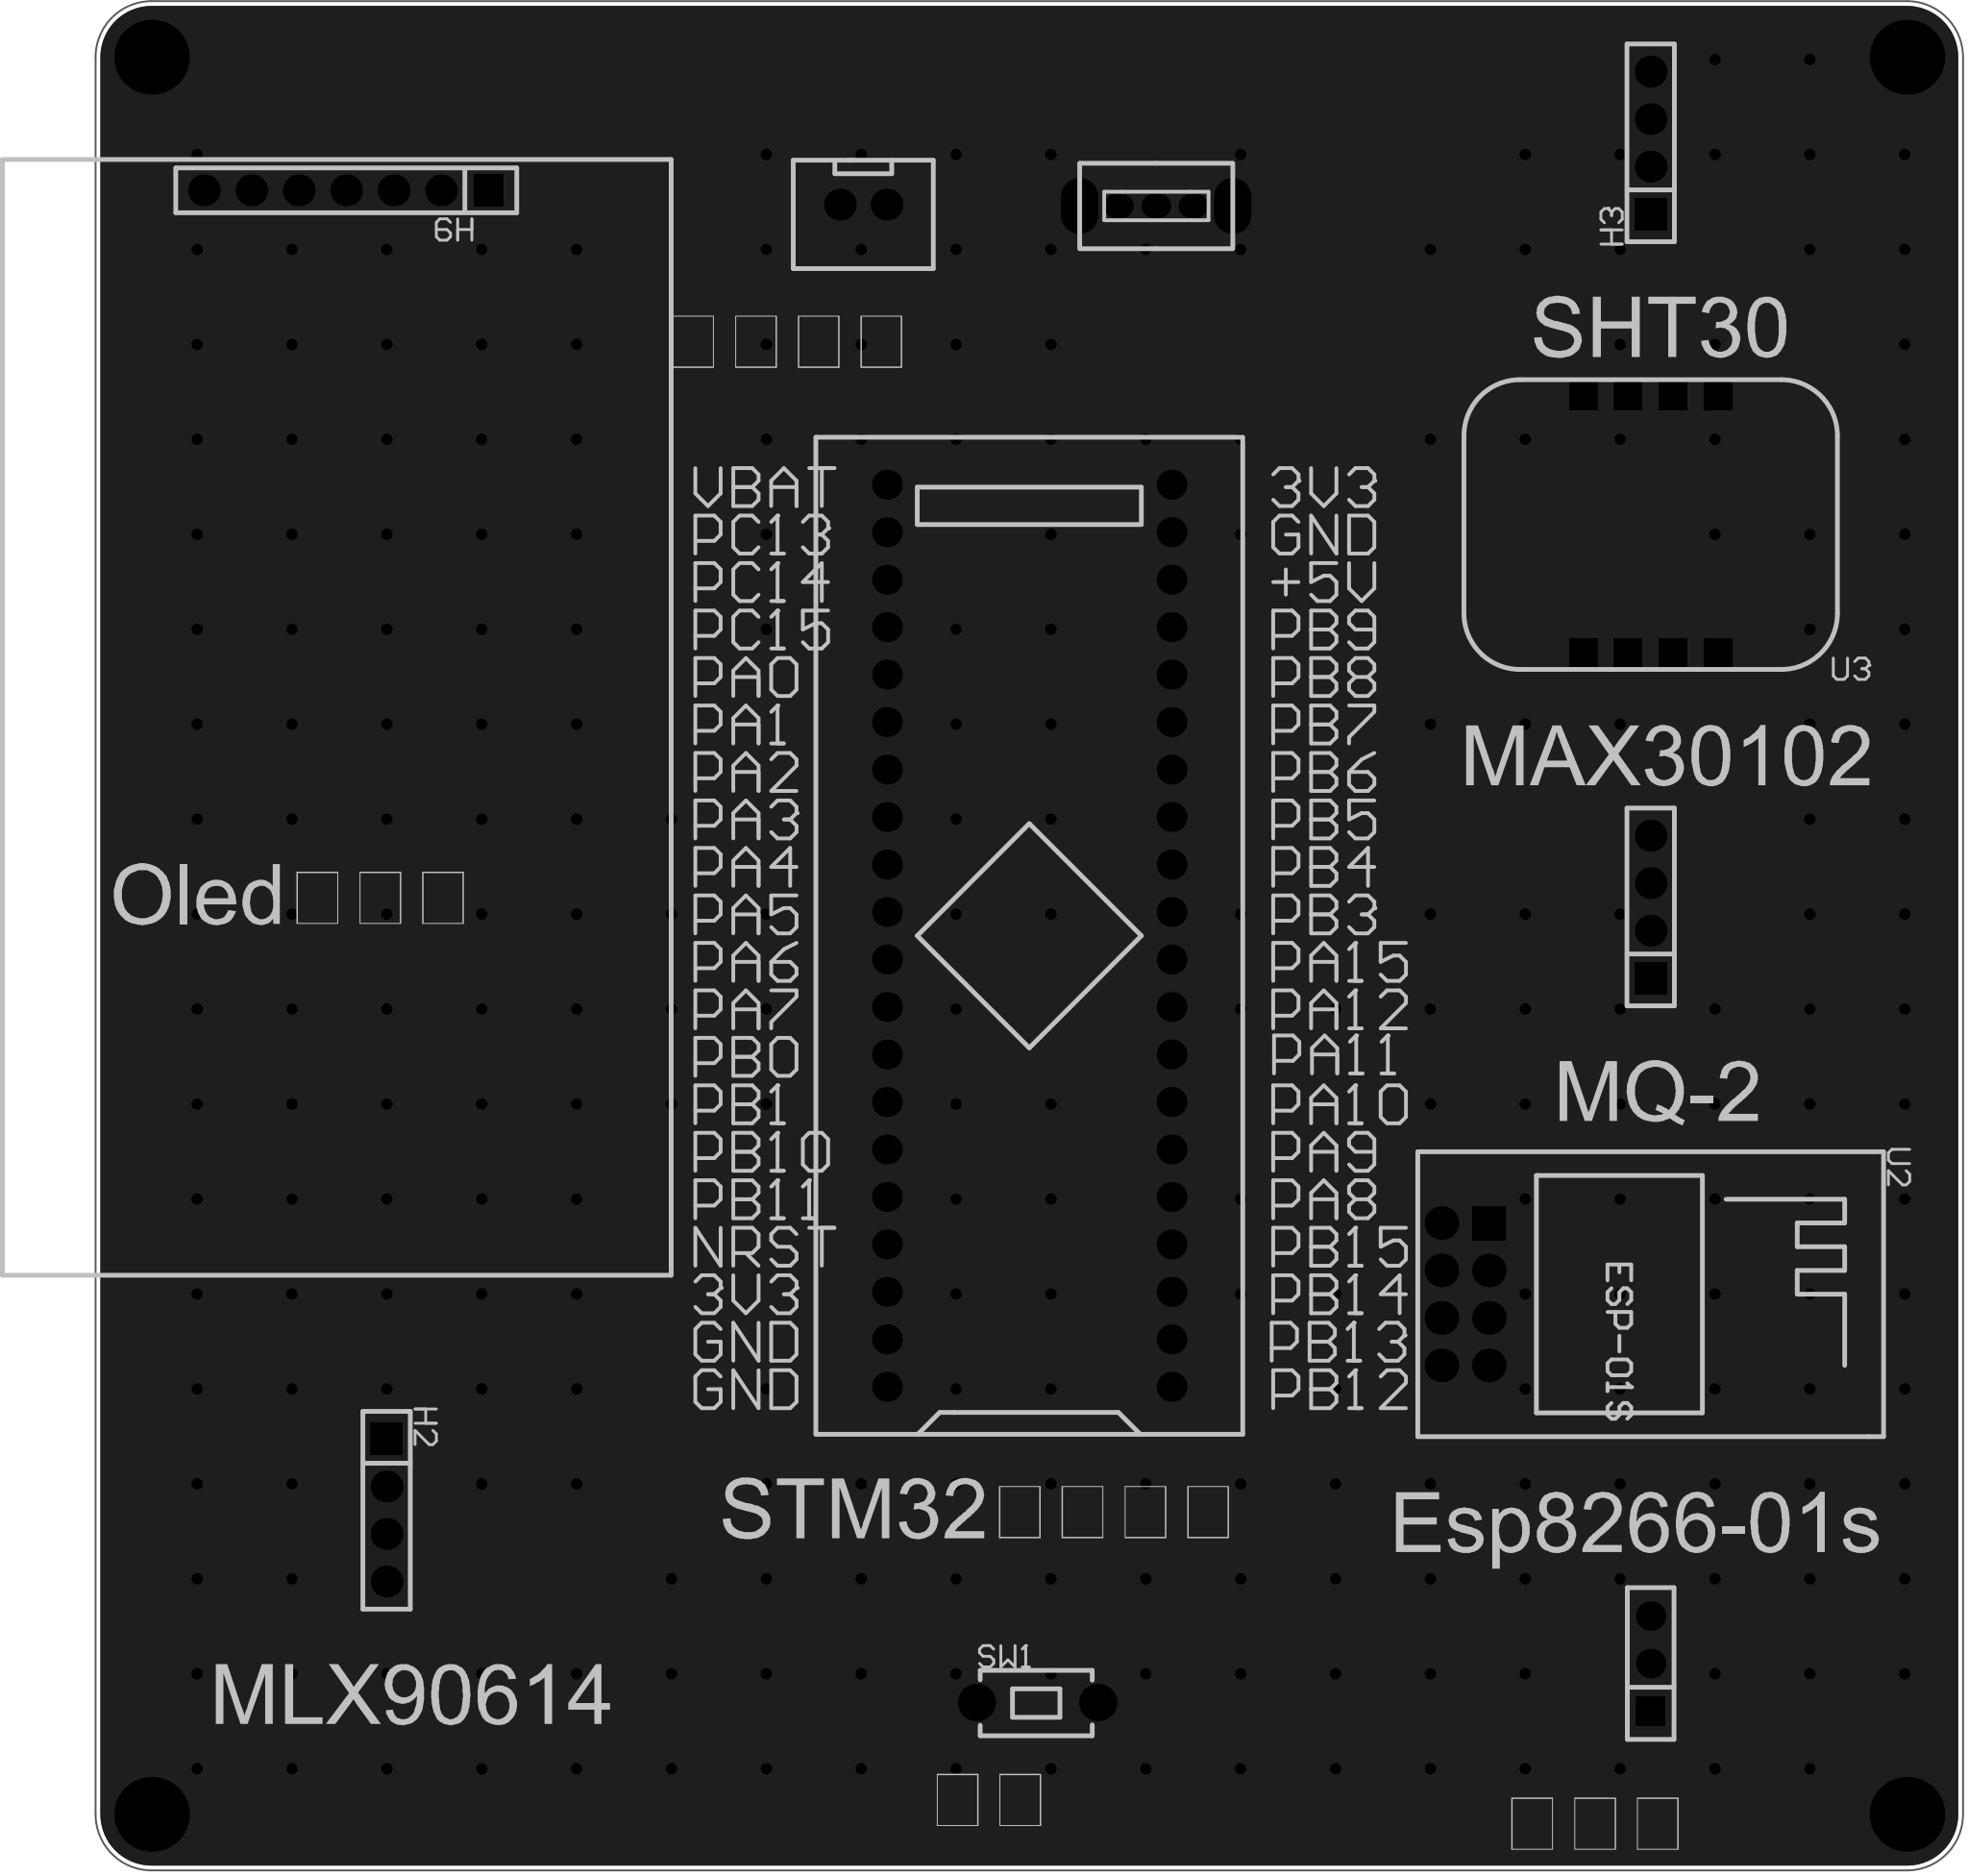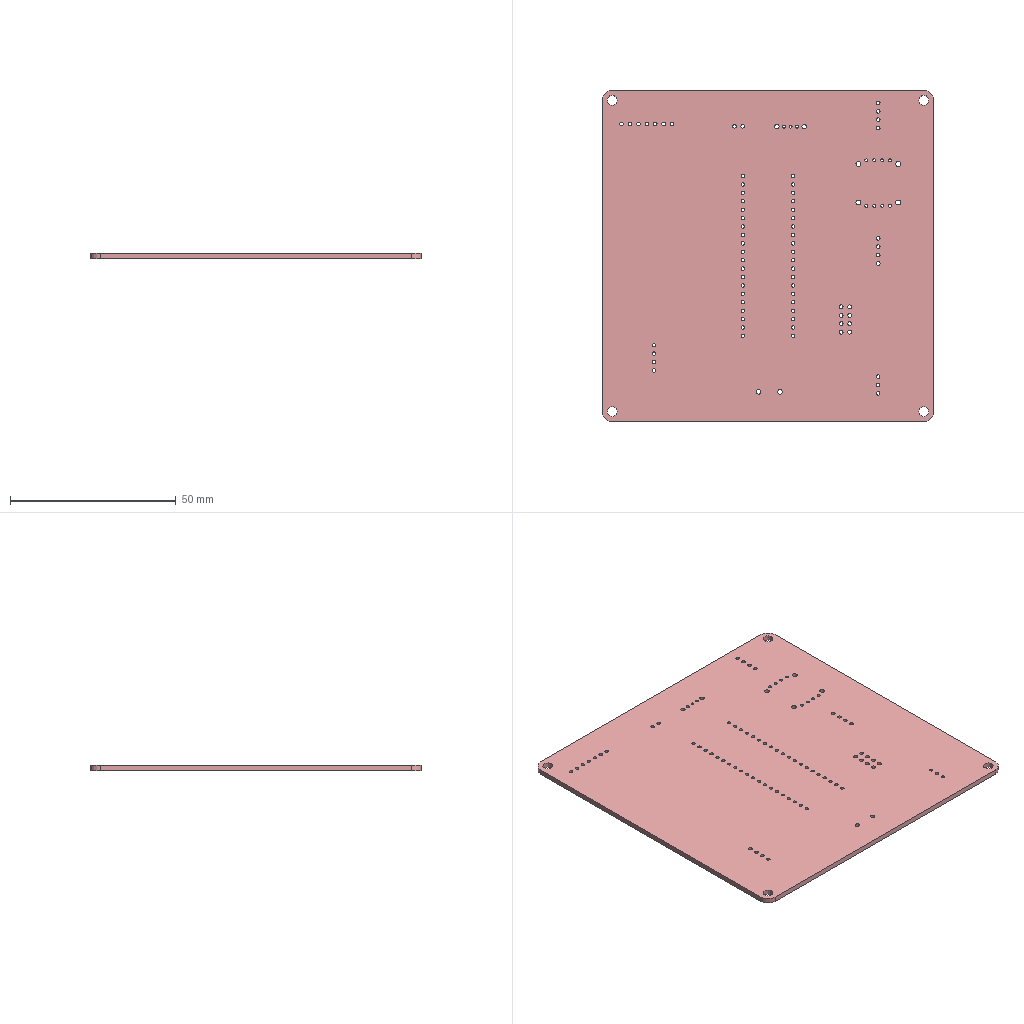Circuit board layout | Altium Designer | box 100 x 100 x 1.6 mm
Layer stack:
# Altium Designer layer stack of  (unit mm; dielectric type: 0 none, 1 core, 2 prepreg, 3 surface material)
index,name,kind,layer,copper_thickness_mm,dielectric_type,dielectric_thickness_mm,dielectric_material,dielectric_constant
0,Top Paste Mask Layer,other,,,,,,
1,Top Silkscreen Layer,other,,,,,,
2,Top Solder Mask Layer,dielectric,,,3,0.01,,3.3
3,Top Layer,copper,Top Layer,0.035,,,,
4,Dielectric1,dielectric,,,3,1.51,FR4,4.5
5,Bottom Layer,copper,Bottom Layer,0.035,,,,
6,Bottom Solder Mask Layer,dielectric,,,3,0.01,,3.3
7,Bottom Silkscreen Layer,other,,,,,,
8,Bottom Paste Mask Layer,other,,,,,,
# drill layer pairs: low layer,high layer
drill_pair,Top Layer,Bottom Layer
Part placement:
Designator,Comment,Layer,Footprint,Center-X(mm),Center-Y(mm),Rotation
U1,STM32F103C8T6-Card,TopLayer,CONN-TH_L53.3-W22.9_STM32F103C8T6-CARD,141.351,130.937,90
CN4,XH2.54*2P_直插,TopLayer,CONN-TH_2P-P2.50-XH2.54-2P,132.461,170.053,0
SW5,,TopLayer,拨动开关,148.148,169.978,180
H1,,TopLayer,HDR-TH_3P-P2.54-V-F,174.625,92.004,90
H4,,TopLayer,HDR-TH_4P-P2.54-V-F,174.625,132.479,90
SW1,,TopLayer,Key_TH_3.5x6x4.3,141.77,89.916,0
H2,,TopLayer,HDR-TH_4P-P2.54-V-F,106.934,100.203,270
H3,,TopLayer,HDR-TH_4P-P2.54-V-F,174.625,173.355,90
H9,,TopLayer,HDR-TH_7P-P2.54-V-F,104.775,170.815,180
U3,MAX30102,TopLayer,MAX30102,174.625,152.933,180
U2,ESP-01S,TopLayer,WIFIM-TH_ESP-01S,164.694,111.763,270
Pad and via stacks:
# Altium Designer via and pad stacks of  (unit mm). Each distinct definition once, with the count of objects using it.
# via: kind,start_layer,end_layer,hole_mm,diameter_mm,mode(0 simple;1 top-mid-bottom;2 full stack),diameter_per_layer,count,example_net
# pad: kind,layer,hole_mm,hole_type(0 round;1 square;2 slot),plating,top_size,top_shape(1 round;2 rect;3 octagon;9 rounded rect),mid_size,bottom_size,mode,footprint,size_per_layer,count,example
pad,Multi-Layer,3,0,plated,4x4,1,4x4,4x4,0,,,4,1
pad,Multi-Layer,1,0,plated,1.6x1.6,1,1.6x1.6,1.6x1.6,0,CONN-TH_L53.3-W22.9_STM32F103C8T6-CARD,,40,U1.1
pad,Multi-Layer,1.05,0,plated,1.7x1.7,1,1.7x1.7,1.7x1.7,0,CONN-TH_2P-P2.50-XH2.54-2P,,2,CN4.2
pad,Multi-Layer,0.8992,0,plated,1.6x1.3,1,1.6x1.3,1.6x1.3,0,\u00B2\u00A6\u00B6\u00AF\u00BF\u00AA\u00B9\u00D8,,3,SW5.1
pad,Multi-Layer,1.3,0,plated,3x1.999,1,3x1.999,3x1.999,0,\u00B2\u00A6\u00B6\u00AF\u00BF\u00AA\u00B9\u00D8,,2,SW5.4
pad,Multi-Layer,1.02,0,plated,1.575x1.575,1,1.575x1.575,1.575x1.575,0,HDR-TH_3P-P2.54-V-F,,2,H1.3
pad,Multi-Layer,1.02,0,plated,1.575x1.575,2,1.575x1.575,1.575x1.575,0,HDR-TH_3P-P2.54-V-F,,1,H1.1
pad,Multi-Layer,1.1,0,plated,1.7x1.7,2,1.7x1.7,1.7x1.7,0,HDR-TH_4P-P2.54-V-F,,3,H4.1
pad,Multi-Layer,1.1,0,plated,1.7x1.7,1,1.7x1.7,1.7x1.7,0,HDR-TH_4P-P2.54-V-F,,9,H4.2
pad,Multi-Layer,1.399,0,plated,1.999x1.999,1,1.999x1.999,1.999x1.999,0,Key_TH_3.5x6x4.3,,2,SW1.A
pad,Multi-Layer,1.1,0,plated,1.7x1.7,1,1.7x1.7,1.7x1.7,0,HDR-TH_7P-P2.54-V-F,,6,H9.7
pad,Multi-Layer,1.1,0,plated,1.575x1.7,2,1.575x1.7,1.575x1.7,0,HDR-TH_7P-P2.54-V-F,,1,H9.1
pad,Multi-Layer,0.9144,0,plated,1.524x1.524,2,1.524x1.524,1.524x1.524,0,MAX30102,,8,U3.1
pad,Multi-Layer,1.2,0,plated,1.8x1.8,2,1.8x1.8,1.8x1.8,0,WIFIM-TH_ESP-01S,,1,U2.1
pad,Multi-Layer,1.2,0,plated,1.8x1.8,1,1.8x1.8,1.8x1.8,0,WIFIM-TH_ESP-01S,,7,U2.2
via,Top Layer,Bottom Layer,0.3048,0.61,0,,256,GND
Copper pours:
name,layer,net,type(0 solid;1 hatched;2 none)
Bottom Layer-GND,Bottom Layer,GND,0
Top Layer-GND,Top Layer,GND,0
Design rules, without the lines most boards share:
# Altium Designer design rules of  (exported by Altium Designer, unit mm)
# columns: name | kind | enabled | priority | scope1 | scope2 | descriptor | typed fields (field=value)
Copper_copperRegion_copperThickness1oz | 0 | disabled | 4 | All | All | Clearance Constraint (Gap=5.984mil) (Disabled)(All),(All) | gap=0.152
Copper_copperRegion_copperThickness1oz_1 | 63 | disabled | 4 | All | All | Board Clearance Constraint (Gap=0mil) (Disabled)(All) |
Copper_copperRegion_Copper_copperRegion | 0 | disabled | 5 | All | All | Clearance Constraint (Gap=5.984mil) (Disabled)(All),(All) | gap=0.152
Copper_copperRegion_Copper_copperRegion_1 | 63 | disabled | 5 | All | All | Board Clearance Constraint (Gap=0mil) (Disabled)(All) |
copperThickness1oz | 0 | enabled | 6 | All | All | Clearance Constraint (Gap=5.984mil) (All),(All) | gap=0.152
copperThickness1oz_1 | 63 | enabled | 6 | All | All | Board Clearance Constraint (Gap=0mil) (All) |
copperRegion_copperThickness1oz | 20 | disabled | 1 | All | All | Polygon Connect Rule(Relief Connect )(Conductor Width=10mil) (Relief Angle=90 Angle) (Entries=4) (Air Gap Width=10mil) (Disabled)(All),(All) | connect_style(0=relief,1=direct,2=none)=0 relief_conductor_width=0.254 relief_entries=4
copperRegion_Copper_copperRegion | 20 | disabled | 2 | All | All | Polygon Connect Rule(Relief Connect )(Conductor Width=10mil) (Relief Angle=90 Angle) (Entries=4) (Air Gap Width=10mil) (Disabled)(All),(All) | connect_style(0=relief,1=direct,2=none)=0 relief_conductor_width=0.254 relief_entries=4
copperRegion | 20 | enabled | 3 | All | All | Polygon Connect Rule(Relief Connect )(Conductor Width=10mil) (Relief Angle=90 Angle) (Entries=4) (Air Gap Width=10mil) (All),(All) | connect_style(0=relief,1=direct,2=none)=0 relief_conductor_width=0.254 relief_entries=4